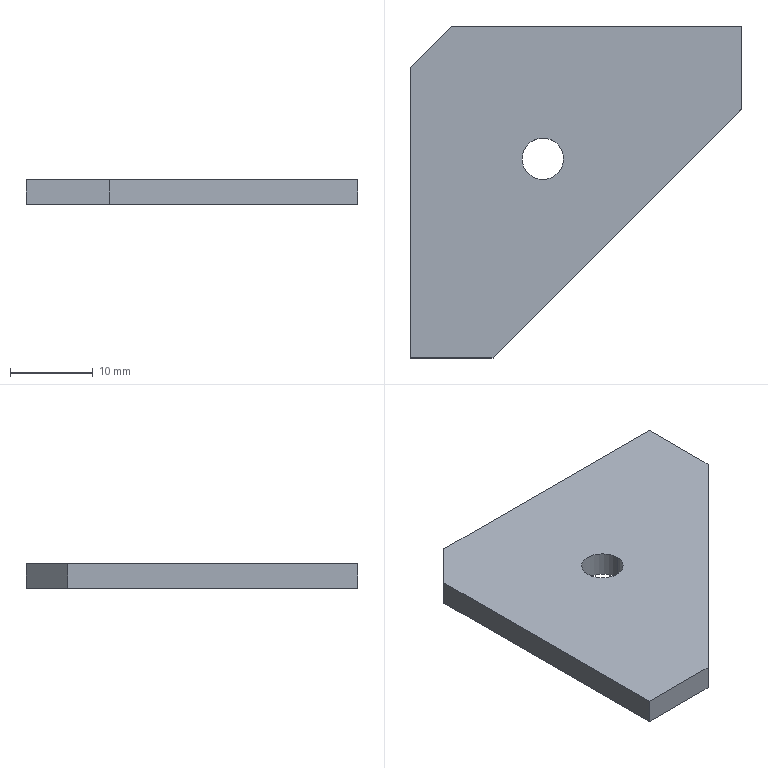Part | SolidWorks | features Chamfer 1, FlatPattern 1, HoleWzd 1, ICE 1, SMBaseFlange 1, SheetMetal 1 | 1 solid | 10 faces | box 40 x 40 x 3 mm | volume 3354 mm3 | plane 8 | cylinder 2 | commonest cylinder face diameters 5 x2
STEP:
#1=CARTESIAN_POINT('',(-6.5,4.,-3.));
#2=VERTEX_POINT('',#1);
#3=CARTESIAN_POINT('',(-1.5,4.,-3.));
#4=VERTEX_POINT('',#3);
#5=CARTESIAN_POINT('',(-4.,4.,-3.));
#6=DIRECTION('',(0.,0.,1.));
#7=DIRECTION('',(1.,0.,0.));
#8=AXIS2_PLACEMENT_3D('',#5,#6,#7);
#9=CIRCLE('',#8,2.5);
#10=EDGE_CURVE('',#2,#4,#9,.T.);
#11=ORIENTED_EDGE('',*,*,#10,.F.);
#12=CARTESIAN_POINT('',(-6.5,4.,0.));
#13=VERTEX_POINT('',#12);
#14=CARTESIAN_POINT('',(-6.5,4.,0.));
#15=DIRECTION('',(0.,0.,1.));
#16=VECTOR('',#15,1000.);
#17=LINE('',#14,#16);
#18=EDGE_CURVE('',#2,#13,#17,.T.);
#19=ORIENTED_EDGE('',*,*,#18,.T.);
#20=CARTESIAN_POINT('',(-1.5,4.,0.));
#21=VERTEX_POINT('',#20);
#22=CARTESIAN_POINT('',(-4.,4.,0.));
#23=DIRECTION('',(0.,0.,1.));
#24=DIRECTION('',(1.,0.,0.));
#25=AXIS2_PLACEMENT_3D('',#22,#23,#24);
#26=CIRCLE('',#25,2.5);
#27=EDGE_CURVE('',#13,#21,#26,.T.);
#28=ORIENTED_EDGE('',*,*,#27,.T.);
#29=CARTESIAN_POINT('',(-1.5,4.,0.));
#30=DIRECTION('',(0.,0.,1.));
#31=VECTOR('',#30,1000.);
#32=LINE('',#29,#31);
#33=EDGE_CURVE('',#4,#21,#32,.T.);
#34=ORIENTED_EDGE('',*,*,#33,.F.);
#35=EDGE_LOOP('',(#11,#19,#28,#34));
#36=FACE_OUTER_BOUND('',#35,.T.);
#37=CARTESIAN_POINT('',(-4.,4.,0.));
#38=DIRECTION('',(0.,0.,1.));
#39=DIRECTION('',(1.,0.,0.));
#40=AXIS2_PLACEMENT_3D('',#37,#38,#39);
#41=CYLINDRICAL_SURFACE('',#40,2.5);
#42=ADVANCED_FACE('',(#36),#41,.F.);
#43=CARTESIAN_POINT('',(20.,10.,0.));
#44=VERTEX_POINT('',#43);
#45=CARTESIAN_POINT('',(20.,20.,0.));
#46=VERTEX_POINT('',#45);
#47=CARTESIAN_POINT('',(20.,20.,0.));
#48=DIRECTION('',(0.,1.,0.));
#49=VECTOR('',#48,1000.);
#50=LINE('',#47,#49);
#51=EDGE_CURVE('',#44,#46,#50,.T.);
#52=ORIENTED_EDGE('',*,*,#51,.F.);
#53=CARTESIAN_POINT('',(20.,10.,-3.));
#54=VERTEX_POINT('',#53);
#55=CARTESIAN_POINT('',(20.,10.,0.));
#56=DIRECTION('',(0.,0.,-1.));
#57=VECTOR('',#56,1000.);
#58=LINE('',#55,#57);
#59=EDGE_CURVE('',#44,#54,#58,.T.);
#60=ORIENTED_EDGE('',*,*,#59,.T.);
#61=CARTESIAN_POINT('',(20.,20.,-3.));
#62=VERTEX_POINT('',#61);
#63=CARTESIAN_POINT('',(20.,20.,-3.));
#64=DIRECTION('',(0.,1.,0.));
#65=VECTOR('',#64,1000.);
#66=LINE('',#63,#65);
#67=EDGE_CURVE('',#54,#62,#66,.T.);
#68=ORIENTED_EDGE('',*,*,#67,.T.);
#69=CARTESIAN_POINT('',(20.,20.,-3.));
#70=DIRECTION('',(0.,0.,1.));
#71=VECTOR('',#70,1000.);
#72=LINE('',#69,#71);
#73=EDGE_CURVE('',#62,#46,#72,.T.);
#74=ORIENTED_EDGE('',*,*,#73,.T.);
#75=EDGE_LOOP('',(#52,#60,#68,#74));
#76=FACE_OUTER_BOUND('',#75,.T.);
#77=CARTESIAN_POINT('',(20.,20.,-3.));
#78=DIRECTION('',(1.,0.,0.));
#79=DIRECTION('',(0.,1.,0.));
#80=AXIS2_PLACEMENT_3D('',#77,#78,#79);
#81=PLANE('',#80);
#82=ADVANCED_FACE('',(#76),#81,.T.);
#83=CARTESIAN_POINT('',(-20.,-20.,-3.));
#84=VERTEX_POINT('',#83);
#85=CARTESIAN_POINT('',(-10.,-20.,-3.));
#86=VERTEX_POINT('',#85);
#87=CARTESIAN_POINT('',(-20.,-20.,-3.));
#88=DIRECTION('',(1.,0.,0.));
#89=VECTOR('',#88,1000.);
#90=LINE('',#87,#89);
#91=EDGE_CURVE('',#84,#86,#90,.T.);
#92=ORIENTED_EDGE('',*,*,#91,.T.);
#93=CARTESIAN_POINT('',(-10.,-20.,0.));
#94=VERTEX_POINT('',#93);
#95=CARTESIAN_POINT('',(-10.,-20.,0.));
#96=DIRECTION('',(0.,0.,-1.));
#97=VECTOR('',#96,1000.);
#98=LINE('',#95,#97);
#99=EDGE_CURVE('',#94,#86,#98,.T.);
#100=ORIENTED_EDGE('',*,*,#99,.F.);
#101=CARTESIAN_POINT('',(-20.,-20.,0.));
#102=VERTEX_POINT('',#101);
#103=CARTESIAN_POINT('',(-20.,-20.,0.));
#104=DIRECTION('',(1.,0.,0.));
#105=VECTOR('',#104,1000.);
#106=LINE('',#103,#105);
#107=EDGE_CURVE('',#102,#94,#106,.T.);
#108=ORIENTED_EDGE('',*,*,#107,.F.);
#109=CARTESIAN_POINT('',(-20.,-20.,-3.));
#110=DIRECTION('',(0.,0.,1.));
#111=VECTOR('',#110,1000.);
#112=LINE('',#109,#111);
#113=EDGE_CURVE('',#84,#102,#112,.T.);
#114=ORIENTED_EDGE('',*,*,#113,.F.);
#115=EDGE_LOOP('',(#92,#100,#108,#114));
#116=FACE_OUTER_BOUND('',#115,.T.);
#117=CARTESIAN_POINT('',(-20.,-20.,-3.));
#118=DIRECTION('',(0.,-1.,0.));
#119=DIRECTION('',(0.,0.,-1.));
#120=AXIS2_PLACEMENT_3D('',#117,#118,#119);
#121=PLANE('',#120);
#122=ADVANCED_FACE('',(#116),#121,.T.);
#123=CARTESIAN_POINT('',(-4.,4.,-3.));
#124=DIRECTION('',(0.,0.,1.));
#125=DIRECTION('',(1.,0.,0.));
#126=AXIS2_PLACEMENT_3D('',#123,#124,#125);
#127=CIRCLE('',#126,2.5);
#128=EDGE_CURVE('',#4,#2,#127,.T.);
#129=ORIENTED_EDGE('',*,*,#128,.T.);
#130=ORIENTED_EDGE('',*,*,#10,.T.);
#131=EDGE_LOOP('',(#129,#130));
#132=FACE_BOUND('',#131,.T.);
#133=CARTESIAN_POINT('',(-10.,-20.,-3.));
#134=DIRECTION('',(-0.7071,-0.7071,0.));
#135=VECTOR('',#134,1000.);
#136=LINE('',#133,#135);
#137=EDGE_CURVE('',#54,#86,#136,.T.);
#138=ORIENTED_EDGE('',*,*,#137,.T.);
#139=ORIENTED_EDGE('',*,*,#91,.F.);
#140=CARTESIAN_POINT('',(-20.,15.,-3.));
#141=VERTEX_POINT('',#140);
#142=CARTESIAN_POINT('',(-20.,20.,-3.));
#143=DIRECTION('',(0.,-1.,0.));
#144=VECTOR('',#143,1000.);
#145=LINE('',#142,#144);
#146=EDGE_CURVE('',#141,#84,#145,.T.);
#147=ORIENTED_EDGE('',*,*,#146,.F.);
#148=CARTESIAN_POINT('',(-15.,20.,-3.));
#149=VERTEX_POINT('',#148);
#150=CARTESIAN_POINT('',(-15.,20.,-3.));
#151=DIRECTION('',(0.7071,0.7071,0.));
#152=VECTOR('',#151,1000.);
#153=LINE('',#150,#152);
#154=EDGE_CURVE('',#141,#149,#153,.T.);
#155=ORIENTED_EDGE('',*,*,#154,.T.);
#156=CARTESIAN_POINT('',(-20.,20.,-3.));
#157=DIRECTION('',(-1.,0.,0.));
#158=VECTOR('',#157,1000.);
#159=LINE('',#156,#158);
#160=EDGE_CURVE('',#62,#149,#159,.T.);
#161=ORIENTED_EDGE('',*,*,#160,.F.);
#162=ORIENTED_EDGE('',*,*,#67,.F.);
#163=EDGE_LOOP('',(#138,#139,#147,#155,#161,#162));
#164=FACE_OUTER_BOUND('',#163,.T.);
#165=CARTESIAN_POINT('',(0.,0.,-3.));
#166=DIRECTION('',(0.,0.,1.));
#167=DIRECTION('',(1.,0.,0.));
#168=AXIS2_PLACEMENT_3D('',#165,#166,#167);
#169=PLANE('',#168);
#170=ADVANCED_FACE('',(#132,#164),#169,.F.);
#171=CARTESIAN_POINT('',(-4.,4.,0.));
#172=DIRECTION('',(0.,0.,1.));
#173=DIRECTION('',(1.,0.,0.));
#174=AXIS2_PLACEMENT_3D('',#171,#172,#173);
#175=CIRCLE('',#174,2.5);
#176=EDGE_CURVE('',#21,#13,#175,.T.);
#177=ORIENTED_EDGE('',*,*,#176,.F.);
#178=ORIENTED_EDGE('',*,*,#27,.F.);
#179=EDGE_LOOP('',(#177,#178));
#180=FACE_BOUND('',#179,.T.);
#181=ORIENTED_EDGE('',*,*,#107,.T.);
#182=CARTESIAN_POINT('',(-10.,-20.,0.));
#183=DIRECTION('',(-0.7071,-0.7071,0.));
#184=VECTOR('',#183,1000.);
#185=LINE('',#182,#184);
#186=EDGE_CURVE('',#44,#94,#185,.T.);
#187=ORIENTED_EDGE('',*,*,#186,.F.);
#188=ORIENTED_EDGE('',*,*,#51,.T.);
#189=CARTESIAN_POINT('',(-15.,20.,0.));
#190=VERTEX_POINT('',#189);
#191=CARTESIAN_POINT('',(-20.,20.,0.));
#192=DIRECTION('',(-1.,0.,0.));
#193=VECTOR('',#192,1000.);
#194=LINE('',#191,#193);
#195=EDGE_CURVE('',#46,#190,#194,.T.);
#196=ORIENTED_EDGE('',*,*,#195,.T.);
#197=CARTESIAN_POINT('',(-20.,15.,0.));
#198=VERTEX_POINT('',#197);
#199=CARTESIAN_POINT('',(-17.5,17.5,0.));
#200=DIRECTION('',(-0.7071,-0.7071,0.));
#201=VECTOR('',#200,1000.);
#202=LINE('',#199,#201);
#203=EDGE_CURVE('',#190,#198,#202,.T.);
#204=ORIENTED_EDGE('',*,*,#203,.T.);
#205=CARTESIAN_POINT('',(-20.,20.,0.));
#206=DIRECTION('',(0.,-1.,0.));
#207=VECTOR('',#206,1000.);
#208=LINE('',#205,#207);
#209=EDGE_CURVE('',#198,#102,#208,.T.);
#210=ORIENTED_EDGE('',*,*,#209,.T.);
#211=EDGE_LOOP('',(#181,#187,#188,#196,#204,#210));
#212=FACE_OUTER_BOUND('',#211,.T.);
#213=CARTESIAN_POINT('',(0.,0.,0.));
#214=DIRECTION('',(0.,0.,1.));
#215=DIRECTION('',(1.,0.,0.));
#216=AXIS2_PLACEMENT_3D('',#213,#214,#215);
#217=PLANE('',#216);
#218=ADVANCED_FACE('',(#180,#212),#217,.T.);
#219=ORIENTED_EDGE('',*,*,#209,.F.);
#220=CARTESIAN_POINT('',(-20.,15.,-3.));
#221=DIRECTION('',(0.,0.,-1.));
#222=VECTOR('',#221,1000.);
#223=LINE('',#220,#222);
#224=EDGE_CURVE('',#198,#141,#223,.T.);
#225=ORIENTED_EDGE('',*,*,#224,.T.);
#226=ORIENTED_EDGE('',*,*,#146,.T.);
#227=ORIENTED_EDGE('',*,*,#113,.T.);
#228=EDGE_LOOP('',(#219,#225,#226,#227));
#229=FACE_OUTER_BOUND('',#228,.T.);
#230=CARTESIAN_POINT('',(-20.,20.,-3.));
#231=DIRECTION('',(-1.,0.,0.));
#232=DIRECTION('',(0.,-1.,0.));
#233=AXIS2_PLACEMENT_3D('',#230,#231,#232);
#234=PLANE('',#233);
#235=ADVANCED_FACE('',(#229),#234,.T.);
#236=ORIENTED_EDGE('',*,*,#160,.T.);
#237=CARTESIAN_POINT('',(-15.,20.,-3.));
#238=DIRECTION('',(0.,0.,1.));
#239=VECTOR('',#238,1000.);
#240=LINE('',#237,#239);
#241=EDGE_CURVE('',#149,#190,#240,.T.);
#242=ORIENTED_EDGE('',*,*,#241,.T.);
#243=ORIENTED_EDGE('',*,*,#195,.F.);
#244=ORIENTED_EDGE('',*,*,#73,.F.);
#245=EDGE_LOOP('',(#236,#242,#243,#244));
#246=FACE_OUTER_BOUND('',#245,.T.);
#247=CARTESIAN_POINT('',(-20.,20.,-3.));
#248=DIRECTION('',(0.,1.,0.));
#249=DIRECTION('',(0.,0.,1.));
#250=AXIS2_PLACEMENT_3D('',#247,#248,#249);
#251=PLANE('',#250);
#252=ADVANCED_FACE('',(#246),#251,.T.);
#253=ORIENTED_EDGE('',*,*,#154,.F.);
#254=ORIENTED_EDGE('',*,*,#224,.F.);
#255=ORIENTED_EDGE('',*,*,#203,.F.);
#256=ORIENTED_EDGE('',*,*,#241,.F.);
#257=EDGE_LOOP('',(#253,#254,#255,#256));
#258=FACE_OUTER_BOUND('',#257,.T.);
#259=CARTESIAN_POINT('',(-15.,20.,-3.));
#260=DIRECTION('',(0.7071,-0.7071,0.));
#261=DIRECTION('',(0.,0.,1.));
#262=AXIS2_PLACEMENT_3D('',#259,#260,#261);
#263=PLANE('',#262);
#264=ADVANCED_FACE('',(#258),#263,.F.);
#265=ORIENTED_EDGE('',*,*,#186,.T.);
#266=ORIENTED_EDGE('',*,*,#99,.T.);
#267=ORIENTED_EDGE('',*,*,#137,.F.);
#268=ORIENTED_EDGE('',*,*,#59,.F.);
#269=EDGE_LOOP('',(#265,#266,#267,#268));
#270=FACE_OUTER_BOUND('',#269,.T.);
#271=CARTESIAN_POINT('',(-10.,-20.,0.));
#272=DIRECTION('',(-0.7071,0.7071,0.));
#273=DIRECTION('',(-0.7071,-0.7071,0.));
#274=AXIS2_PLACEMENT_3D('',#271,#272,#273);
#275=PLANE('',#274);
#276=ADVANCED_FACE('',(#270),#275,.F.);
#277=ORIENTED_EDGE('',*,*,#18,.F.);
#278=ORIENTED_EDGE('',*,*,#128,.F.);
#279=ORIENTED_EDGE('',*,*,#33,.T.);
#280=ORIENTED_EDGE('',*,*,#176,.T.);
#281=EDGE_LOOP('',(#277,#278,#279,#280));
#282=FACE_OUTER_BOUND('',#281,.T.);
#283=CARTESIAN_POINT('',(-4.,4.,0.));
#284=DIRECTION('',(0.,0.,1.));
#285=DIRECTION('',(1.,0.,0.));
#286=AXIS2_PLACEMENT_3D('',#283,#284,#285);
#287=CYLINDRICAL_SURFACE('',#286,2.5);
#288=ADVANCED_FACE('',(#282),#287,.F.);
#289=CLOSED_SHELL('',(#42,#82,#122,#170,#218,#235,#252,#264,#276,#288));
#290=MANIFOLD_SOLID_BREP('',#289);
#291=CARTESIAN_POINT('',(0.,0.,0.));
#292=DIRECTION('',(0.,0.,1.));
#293=DIRECTION('',(1.,0.,0.));
#294=AXIS2_PLACEMENT_3D('',#291,#292,#293);
#295=(LENGTH_UNIT()NAMED_UNIT(*)SI_UNIT(.MILLI.,.METRE.));
#296=UNCERTAINTY_MEASURE_WITH_UNIT(LENGTH_MEASURE(0.00001),#295,'','');
#297=(NAMED_UNIT(*)PLANE_ANGLE_UNIT()SI_UNIT($,.RADIAN.));
#298=(NAMED_UNIT(*)SI_UNIT($,.STERADIAN.)SOLID_ANGLE_UNIT());
#299=(GEOMETRIC_REPRESENTATION_CONTEXT(3)GLOBAL_UNCERTAINTY_ASSIGNED_CONTEXT((#296))GLOBAL_UNIT_ASSIGNED_CONTEXT((#295,#297,#298))REPRESENTATION_CONTEXT('',''));
#300=ADVANCED_BREP_SHAPE_REPRESENTATION('',(#290,#294),#299);